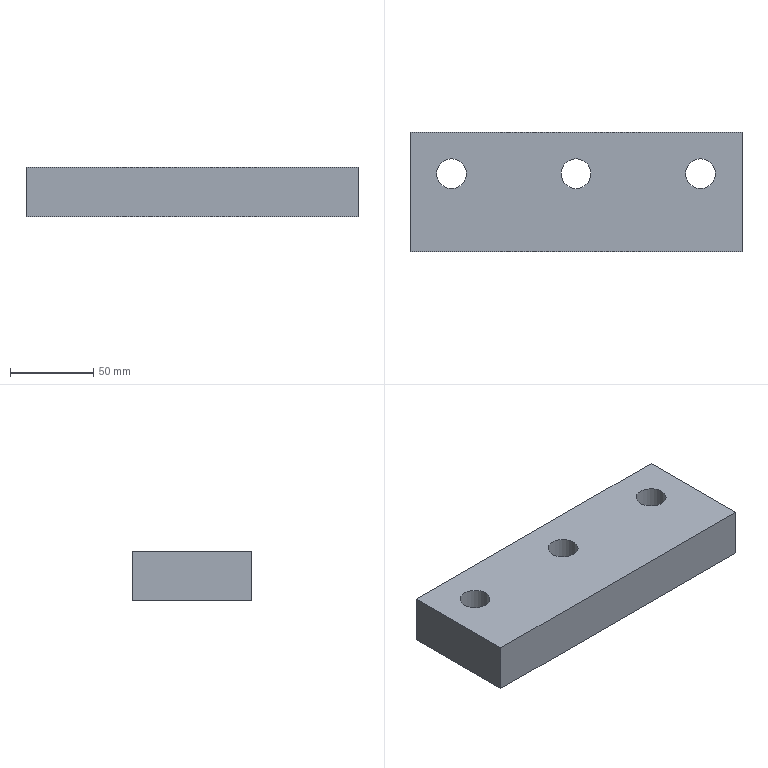Part | NX | features solid 2 | 1 solid | 9 faces | box 200 x 72 x 30 mm | volume 409098 mm3 | plane 6 | cylinder 3 | commonest cylinder face diameters 18 x3
STEP:
#1=CARTESIAN_POINT('',(210.,378.,140.));
#2=VERTEX_POINT('',#1);
#3=CARTESIAN_POINT('',(210.,387.,140.));
#4=DIRECTION('',(0.,0.,1.));
#5=DIRECTION('',(0.,-1.,0.));
#6=AXIS2_PLACEMENT_3D('',#3,#4,#5);
#7=CIRCLE('',#6,9.);
#8=EDGE_CURVE('',#2,#2,#7,.T.);
#9=ORIENTED_EDGE('',*,*,#8,.F.);
#10=EDGE_LOOP('',(#9));
#11=FACE_BOUND('',#10,.T.);
#12=CARTESIAN_POINT('',(285.,378.,140.));
#13=VERTEX_POINT('',#12);
#14=CARTESIAN_POINT('',(285.,387.,140.));
#15=DIRECTION('',(0.,0.,1.));
#16=DIRECTION('',(0.,-1.,0.));
#17=AXIS2_PLACEMENT_3D('',#14,#15,#16);
#18=CIRCLE('',#17,9.);
#19=EDGE_CURVE('',#13,#13,#18,.T.);
#20=ORIENTED_EDGE('',*,*,#19,.F.);
#21=EDGE_LOOP('',(#20));
#22=FACE_BOUND('',#21,.T.);
#23=CARTESIAN_POINT('',(135.,378.,140.));
#24=VERTEX_POINT('',#23);
#25=CARTESIAN_POINT('',(135.,387.,140.));
#26=DIRECTION('',(0.,0.,1.));
#27=DIRECTION('',(0.,-1.,0.));
#28=AXIS2_PLACEMENT_3D('',#25,#26,#27);
#29=CIRCLE('',#28,9.);
#30=EDGE_CURVE('',#24,#24,#29,.T.);
#31=ORIENTED_EDGE('',*,*,#30,.F.);
#32=EDGE_LOOP('',(#31));
#33=FACE_BOUND('',#32,.T.);
#34=CARTESIAN_POINT('',(110.,412.,140.));
#35=VERTEX_POINT('',#34);
#36=CARTESIAN_POINT('',(110.,340.,140.));
#37=VERTEX_POINT('',#36);
#38=CARTESIAN_POINT('',(110.,402.,140.));
#39=DIRECTION('',(0.,-1.,0.));
#40=VECTOR('',#39,1000.);
#41=LINE('',#38,#40);
#42=EDGE_CURVE('',#35,#37,#41,.T.);
#43=ORIENTED_EDGE('',*,*,#42,.T.);
#44=CARTESIAN_POINT('',(310.,340.,140.));
#45=VERTEX_POINT('',#44);
#46=CARTESIAN_POINT('',(110.,340.,140.));
#47=DIRECTION('',(1.,0.,0.));
#48=VECTOR('',#47,1000.);
#49=LINE('',#46,#48);
#50=EDGE_CURVE('',#37,#45,#49,.T.);
#51=ORIENTED_EDGE('',*,*,#50,.T.);
#52=CARTESIAN_POINT('',(310.,412.,140.));
#53=VERTEX_POINT('',#52);
#54=CARTESIAN_POINT('',(310.,332.,140.));
#55=DIRECTION('',(0.,1.,0.));
#56=VECTOR('',#55,1000.);
#57=LINE('',#54,#56);
#58=EDGE_CURVE('',#53,#45,#57,.F.);
#59=ORIENTED_EDGE('',*,*,#58,.F.);
#60=CARTESIAN_POINT('',(110.,412.,140.));
#61=DIRECTION('',(1.,0.,0.));
#62=VECTOR('',#61,1000.);
#63=LINE('',#60,#62);
#64=EDGE_CURVE('',#35,#53,#63,.T.);
#65=ORIENTED_EDGE('',*,*,#64,.F.);
#66=EDGE_LOOP('',(#43,#51,#59,#65));
#67=FACE_BOUND('',#66,.T.);
#68=CARTESIAN_POINT('',(110.,402.,140.));
#69=DIRECTION('',(0.,0.,1.));
#70=DIRECTION('',(1.,0.,0.));
#71=AXIS2_PLACEMENT_3D('',#68,#69,#70);
#72=PLANE('',#71);
#73=ADVANCED_FACE('',(#11,#22,#33,#67),#72,.T.);
#74=ORIENTED_EDGE('',*,*,#58,.T.);
#75=CARTESIAN_POINT('',(310.,340.,110.));
#76=VERTEX_POINT('',#75);
#77=CARTESIAN_POINT('',(310.,340.,190.));
#78=DIRECTION('',(0.,0.,1.));
#79=VECTOR('',#78,1000.);
#80=LINE('',#77,#79);
#81=EDGE_CURVE('',#45,#76,#80,.F.);
#82=ORIENTED_EDGE('',*,*,#81,.T.);
#83=CARTESIAN_POINT('',(310.,412.,110.));
#84=VERTEX_POINT('',#83);
#85=CARTESIAN_POINT('',(310.,402.,110.));
#86=DIRECTION('',(0.,-1.,0.));
#87=VECTOR('',#86,1000.);
#88=LINE('',#85,#87);
#89=EDGE_CURVE('',#84,#76,#88,.T.);
#90=ORIENTED_EDGE('',*,*,#89,.F.);
#91=CARTESIAN_POINT('',(310.,412.,190.));
#92=DIRECTION('',(0.,0.,1.));
#93=VECTOR('',#92,1000.);
#94=LINE('',#91,#93);
#95=EDGE_CURVE('',#53,#84,#94,.F.);
#96=ORIENTED_EDGE('',*,*,#95,.F.);
#97=EDGE_LOOP('',(#74,#82,#90,#96));
#98=FACE_BOUND('',#97,.T.);
#99=CARTESIAN_POINT('',(310.,332.,190.));
#100=DIRECTION('',(-1.,0.,0.));
#101=DIRECTION('',(0.,0.,-1.));
#102=AXIS2_PLACEMENT_3D('',#99,#100,#101);
#103=PLANE('',#102);
#104=ADVANCED_FACE('',(#98),#103,.F.);
#105=CARTESIAN_POINT('',(210.,378.,110.));
#106=VERTEX_POINT('',#105);
#107=CARTESIAN_POINT('',(210.,387.,110.));
#108=DIRECTION('',(0.,0.,1.));
#109=DIRECTION('',(0.,-1.,0.));
#110=AXIS2_PLACEMENT_3D('',#107,#108,#109);
#111=CIRCLE('',#110,9.);
#112=EDGE_CURVE('',#106,#106,#111,.T.);
#113=ORIENTED_EDGE('',*,*,#112,.T.);
#114=EDGE_LOOP('',(#113));
#115=FACE_BOUND('',#114,.T.);
#116=CARTESIAN_POINT('',(285.,378.,110.));
#117=VERTEX_POINT('',#116);
#118=CARTESIAN_POINT('',(285.,387.,110.));
#119=DIRECTION('',(0.,0.,1.));
#120=DIRECTION('',(0.,-1.,0.));
#121=AXIS2_PLACEMENT_3D('',#118,#119,#120);
#122=CIRCLE('',#121,9.);
#123=EDGE_CURVE('',#117,#117,#122,.T.);
#124=ORIENTED_EDGE('',*,*,#123,.T.);
#125=EDGE_LOOP('',(#124));
#126=FACE_BOUND('',#125,.T.);
#127=CARTESIAN_POINT('',(135.,378.,110.));
#128=VERTEX_POINT('',#127);
#129=CARTESIAN_POINT('',(135.,387.,110.));
#130=DIRECTION('',(0.,0.,1.));
#131=DIRECTION('',(0.,-1.,0.));
#132=AXIS2_PLACEMENT_3D('',#129,#130,#131);
#133=CIRCLE('',#132,9.);
#134=EDGE_CURVE('',#128,#128,#133,.T.);
#135=ORIENTED_EDGE('',*,*,#134,.T.);
#136=EDGE_LOOP('',(#135));
#137=FACE_BOUND('',#136,.T.);
#138=ORIENTED_EDGE('',*,*,#89,.T.);
#139=CARTESIAN_POINT('',(110.,340.,110.));
#140=VERTEX_POINT('',#139);
#141=CARTESIAN_POINT('',(110.,340.,110.));
#142=DIRECTION('',(-1.,0.,0.));
#143=VECTOR('',#142,1000.);
#144=LINE('',#141,#143);
#145=EDGE_CURVE('',#140,#76,#144,.F.);
#146=ORIENTED_EDGE('',*,*,#145,.F.);
#147=CARTESIAN_POINT('',(110.,412.,110.));
#148=VERTEX_POINT('',#147);
#149=CARTESIAN_POINT('',(110.,332.,110.));
#150=DIRECTION('',(0.,1.,0.));
#151=VECTOR('',#150,1000.);
#152=LINE('',#149,#151);
#153=EDGE_CURVE('',#148,#140,#152,.F.);
#154=ORIENTED_EDGE('',*,*,#153,.F.);
#155=CARTESIAN_POINT('',(110.,412.,110.));
#156=DIRECTION('',(-1.,0.,0.));
#157=VECTOR('',#156,1000.);
#158=LINE('',#155,#157);
#159=EDGE_CURVE('',#148,#84,#158,.F.);
#160=ORIENTED_EDGE('',*,*,#159,.T.);
#161=EDGE_LOOP('',(#138,#146,#154,#160));
#162=FACE_BOUND('',#161,.T.);
#163=CARTESIAN_POINT('',(110.,402.,110.));
#164=DIRECTION('',(0.,0.,1.));
#165=DIRECTION('',(1.,0.,0.));
#166=AXIS2_PLACEMENT_3D('',#163,#164,#165);
#167=PLANE('',#166);
#168=ADVANCED_FACE('',(#115,#126,#137,#162),#167,.F.);
#169=CARTESIAN_POINT('',(110.,412.,140.));
#170=DIRECTION('',(0.,0.,-1.));
#171=VECTOR('',#170,1000.);
#172=LINE('',#169,#171);
#173=EDGE_CURVE('',#35,#148,#172,.T.);
#174=ORIENTED_EDGE('',*,*,#173,.T.);
#175=ORIENTED_EDGE('',*,*,#153,.T.);
#176=CARTESIAN_POINT('',(110.,340.,140.));
#177=DIRECTION('',(0.,0.,-1.));
#178=VECTOR('',#177,1000.);
#179=LINE('',#176,#178);
#180=EDGE_CURVE('',#37,#140,#179,.T.);
#181=ORIENTED_EDGE('',*,*,#180,.F.);
#182=ORIENTED_EDGE('',*,*,#42,.F.);
#183=EDGE_LOOP('',(#174,#175,#181,#182));
#184=FACE_BOUND('',#183,.T.);
#185=CARTESIAN_POINT('',(110.,332.,190.));
#186=DIRECTION('',(-1.,0.,0.));
#187=DIRECTION('',(0.,0.,-1.));
#188=AXIS2_PLACEMENT_3D('',#185,#186,#187);
#189=PLANE('',#188);
#190=ADVANCED_FACE('',(#184),#189,.T.);
#191=ORIENTED_EDGE('',*,*,#145,.T.);
#192=ORIENTED_EDGE('',*,*,#81,.F.);
#193=ORIENTED_EDGE('',*,*,#50,.F.);
#194=ORIENTED_EDGE('',*,*,#180,.T.);
#195=EDGE_LOOP('',(#191,#192,#193,#194));
#196=FACE_BOUND('',#195,.T.);
#197=CARTESIAN_POINT('',(110.,340.,140.));
#198=DIRECTION('',(0.,-1.,0.));
#199=DIRECTION('',(0.,0.,1.));
#200=AXIS2_PLACEMENT_3D('',#197,#198,#199);
#201=PLANE('',#200);
#202=ADVANCED_FACE('',(#196),#201,.T.);
#203=ORIENTED_EDGE('',*,*,#159,.F.);
#204=ORIENTED_EDGE('',*,*,#173,.F.);
#205=ORIENTED_EDGE('',*,*,#64,.T.);
#206=ORIENTED_EDGE('',*,*,#95,.T.);
#207=EDGE_LOOP('',(#203,#204,#205,#206));
#208=FACE_BOUND('',#207,.T.);
#209=CARTESIAN_POINT('',(110.,412.,140.));
#210=DIRECTION('',(0.,-1.,0.));
#211=DIRECTION('',(0.,0.,1.));
#212=AXIS2_PLACEMENT_3D('',#209,#210,#211);
#213=PLANE('',#212);
#214=ADVANCED_FACE('',(#208),#213,.F.);
#215=ORIENTED_EDGE('',*,*,#30,.T.);
#216=EDGE_LOOP('',(#215));
#217=FACE_BOUND('',#216,.T.);
#218=ORIENTED_EDGE('',*,*,#134,.F.);
#219=EDGE_LOOP('',(#218));
#220=FACE_BOUND('',#219,.T.);
#221=CARTESIAN_POINT('',(135.,387.,120.));
#222=DIRECTION('',(0.,0.,1.));
#223=DIRECTION('',(0.,-1.,0.));
#224=AXIS2_PLACEMENT_3D('',#221,#222,#223);
#225=CYLINDRICAL_SURFACE('',#224,9.);
#226=ADVANCED_FACE('',(#217,#220),#225,.F.);
#227=ORIENTED_EDGE('',*,*,#19,.T.);
#228=EDGE_LOOP('',(#227));
#229=FACE_BOUND('',#228,.T.);
#230=ORIENTED_EDGE('',*,*,#123,.F.);
#231=EDGE_LOOP('',(#230));
#232=FACE_BOUND('',#231,.T.);
#233=CARTESIAN_POINT('',(285.,387.,120.));
#234=DIRECTION('',(0.,0.,1.));
#235=DIRECTION('',(0.,-1.,0.));
#236=AXIS2_PLACEMENT_3D('',#233,#234,#235);
#237=CYLINDRICAL_SURFACE('',#236,9.);
#238=ADVANCED_FACE('',(#229,#232),#237,.F.);
#239=ORIENTED_EDGE('',*,*,#8,.T.);
#240=EDGE_LOOP('',(#239));
#241=FACE_BOUND('',#240,.T.);
#242=ORIENTED_EDGE('',*,*,#112,.F.);
#243=EDGE_LOOP('',(#242));
#244=FACE_BOUND('',#243,.T.);
#245=CARTESIAN_POINT('',(210.,387.,120.));
#246=DIRECTION('',(0.,0.,1.));
#247=DIRECTION('',(0.,-1.,0.));
#248=AXIS2_PLACEMENT_3D('',#245,#246,#247);
#249=CYLINDRICAL_SURFACE('',#248,9.);
#250=ADVANCED_FACE('',(#241,#244),#249,.F.);
#251=CLOSED_SHELL('',(#73,#104,#168,#190,#202,#214,#226,#238,#250));
#252=MANIFOLD_SOLID_BREP('',#251);
#253=(LENGTH_UNIT()NAMED_UNIT(*)SI_UNIT(.MILLI.,.METRE.));
#254=UNCERTAINTY_MEASURE_WITH_UNIT(LENGTH_MEASURE(0.00001),#253,'','');
#255=(NAMED_UNIT(*)PLANE_ANGLE_UNIT()SI_UNIT($,.RADIAN.));
#256=(NAMED_UNIT(*)SI_UNIT($,.STERADIAN.)SOLID_ANGLE_UNIT());
#257=(GEOMETRIC_REPRESENTATION_CONTEXT(3)GLOBAL_UNCERTAINTY_ASSIGNED_CONTEXT((#254))GLOBAL_UNIT_ASSIGNED_CONTEXT((#253,#255,#256))REPRESENTATION_CONTEXT('',''));
#258=ADVANCED_BREP_SHAPE_REPRESENTATION('',(#252),#257);